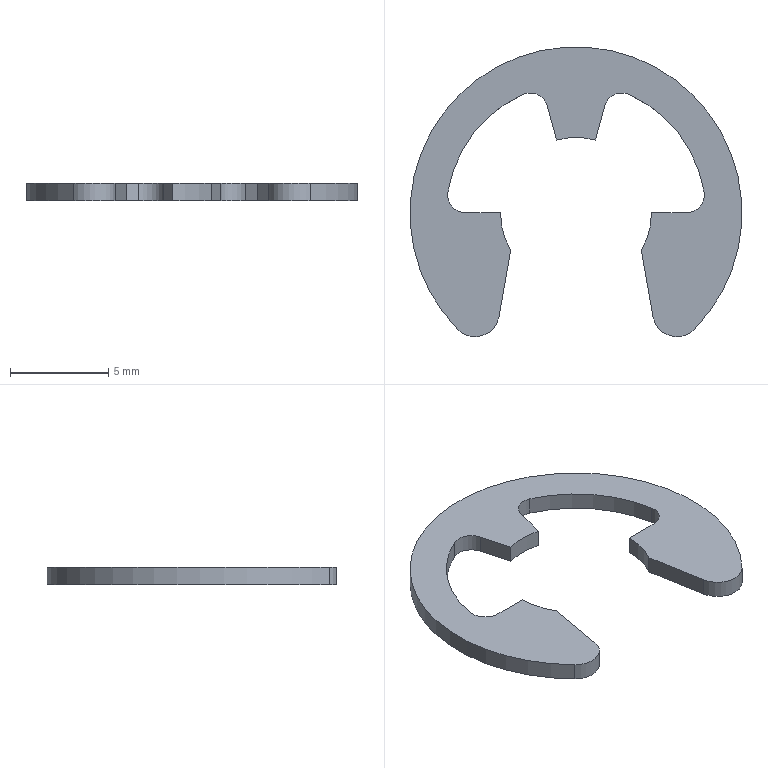Part | SolidWorks | features BaseBody 1 | 1 solid | 20 faces | box 16.932 x 14.78 x 0.889 mm | volume 89.694 mm3 | cylinder 12 | plane 8 | commonest cylinder face diameters 1.829 x4 7.696 x3 2.475 x2 13.237 x2 16.932 x1
STEP:
#1=CARTESIAN_POINT('',(5.631,0.,0.));
#2=VERTEX_POINT('',#1);
#3=CARTESIAN_POINT('',(6.533,1.061,0.));
#4=VERTEX_POINT('',#3);
#5=CARTESIAN_POINT('',(5.631,0.9143,0.));
#6=DIRECTION('',(0.,0.,1.));
#7=DIRECTION('',(0.,-1.,0.));
#8=AXIS2_PLACEMENT_3D('',#5,#6,#7);
#9=CIRCLE('',#8,0.9143);
#10=EDGE_CURVE('',#2,#4,#9,.T.);
#11=ORIENTED_EDGE('',*,*,#10,.F.);
#12=CARTESIAN_POINT('',(3.848,0.,0.));
#13=VERTEX_POINT('',#12);
#14=CARTESIAN_POINT('',(3.848,0.,0.));
#15=DIRECTION('',(1.,0.,0.));
#16=VECTOR('',#15,1000.);
#17=LINE('',#14,#16);
#18=EDGE_CURVE('',#13,#2,#17,.T.);
#19=ORIENTED_EDGE('',*,*,#18,.F.);
#20=CARTESIAN_POINT('',(3.333,-1.924,0.));
#21=VERTEX_POINT('',#20);
#22=CARTESIAN_POINT('',(0.,0.,0.));
#23=DIRECTION('',(0.,0.,1.));
#24=DIRECTION('',(0.866,-0.5,0.));
#25=AXIS2_PLACEMENT_3D('',#22,#23,#24);
#26=CIRCLE('',#25,3.848);
#27=EDGE_CURVE('',#21,#13,#26,.T.);
#28=ORIENTED_EDGE('',*,*,#27,.F.);
#29=CARTESIAN_POINT('',(3.926,-5.292,0.));
#30=VERTEX_POINT('',#29);
#31=CARTESIAN_POINT('',(3.926,-5.292,0.));
#32=DIRECTION('',(-0.1736,0.9848,0.));
#33=VECTOR('',#32,1000.);
#34=LINE('',#31,#33);
#35=EDGE_CURVE('',#30,#21,#34,.T.);
#36=ORIENTED_EDGE('',*,*,#35,.F.);
#37=CARTESIAN_POINT('',(6.026,-5.946,0.));
#38=VERTEX_POINT('',#37);
#39=CARTESIAN_POINT('',(5.145,-5.077,0.));
#40=DIRECTION('',(0.,0.,-1.));
#41=DIRECTION('',(0.7118,-0.7024,0.));
#42=AXIS2_PLACEMENT_3D('',#39,#40,#41);
#43=CIRCLE('',#42,1.238);
#44=EDGE_CURVE('',#38,#30,#43,.T.);
#45=ORIENTED_EDGE('',*,*,#44,.F.);
#46=CARTESIAN_POINT('',(-6.026,-5.946,0.));
#47=VERTEX_POINT('',#46);
#48=CARTESIAN_POINT('',(0.,0.,0.));
#49=DIRECTION('',(0.,0.,-1.));
#50=DIRECTION('',(-0.7118,-0.7024,0.));
#51=AXIS2_PLACEMENT_3D('',#48,#49,#50);
#52=CIRCLE('',#51,8.466);
#53=EDGE_CURVE('',#47,#38,#52,.T.);
#54=ORIENTED_EDGE('',*,*,#53,.F.);
#55=CARTESIAN_POINT('',(-3.926,-5.292,0.));
#56=VERTEX_POINT('',#55);
#57=CARTESIAN_POINT('',(-5.145,-5.077,0.));
#58=DIRECTION('',(0.,0.,-1.));
#59=DIRECTION('',(0.9848,-0.1736,0.));
#60=AXIS2_PLACEMENT_3D('',#57,#58,#59);
#61=CIRCLE('',#60,1.238);
#62=EDGE_CURVE('',#56,#47,#61,.T.);
#63=ORIENTED_EDGE('',*,*,#62,.F.);
#64=CARTESIAN_POINT('',(-3.333,-1.924,0.));
#65=VERTEX_POINT('',#64);
#66=CARTESIAN_POINT('',(-3.333,-1.924,0.));
#67=DIRECTION('',(-0.1736,-0.9848,0.));
#68=VECTOR('',#67,1000.);
#69=LINE('',#66,#68);
#70=EDGE_CURVE('',#65,#56,#69,.T.);
#71=ORIENTED_EDGE('',*,*,#70,.F.);
#72=CARTESIAN_POINT('',(-3.848,0.,0.));
#73=VERTEX_POINT('',#72);
#74=CARTESIAN_POINT('',(0.,0.,0.));
#75=DIRECTION('',(0.,0.,1.));
#76=DIRECTION('',(-1.,0.,0.));
#77=AXIS2_PLACEMENT_3D('',#74,#75,#76);
#78=CIRCLE('',#77,3.848);
#79=EDGE_CURVE('',#73,#65,#78,.T.);
#80=ORIENTED_EDGE('',*,*,#79,.F.);
#81=CARTESIAN_POINT('',(-5.631,0.,0.));
#82=VERTEX_POINT('',#81);
#83=CARTESIAN_POINT('',(-5.631,0.,0.));
#84=DIRECTION('',(1.,0.,0.));
#85=VECTOR('',#84,1000.);
#86=LINE('',#83,#85);
#87=EDGE_CURVE('',#82,#73,#86,.T.);
#88=ORIENTED_EDGE('',*,*,#87,.F.);
#89=CARTESIAN_POINT('',(-6.533,1.061,0.));
#90=VERTEX_POINT('',#89);
#91=CARTESIAN_POINT('',(-5.631,0.9143,0.));
#92=DIRECTION('',(0.,0.,1.));
#93=DIRECTION('',(-0.9871,0.1603,0.));
#94=AXIS2_PLACEMENT_3D('',#91,#92,#93);
#95=CIRCLE('',#94,0.9143);
#96=EDGE_CURVE('',#90,#82,#95,.T.);
#97=ORIENTED_EDGE('',*,*,#96,.F.);
#98=CARTESIAN_POINT('',(-2.716,6.036,0.));
#99=VERTEX_POINT('',#98);
#100=CARTESIAN_POINT('',(0.,0.,0.));
#101=DIRECTION('',(0.,0.,1.));
#102=DIRECTION('',(-0.4103,0.912,0.));
#103=AXIS2_PLACEMENT_3D('',#100,#101,#102);
#104=CIRCLE('',#103,6.619);
#105=EDGE_CURVE('',#99,#90,#104,.T.);
#106=ORIENTED_EDGE('',*,*,#105,.F.);
#107=CARTESIAN_POINT('',(-1.457,5.439,0.));
#108=VERTEX_POINT('',#107);
#109=CARTESIAN_POINT('',(-2.34,5.202,0.));
#110=DIRECTION('',(0.,0.,1.));
#111=DIRECTION('',(0.9659,0.2588,0.));
#112=AXIS2_PLACEMENT_3D('',#109,#110,#111);
#113=CIRCLE('',#112,0.9143);
#114=EDGE_CURVE('',#108,#99,#113,.T.);
#115=ORIENTED_EDGE('',*,*,#114,.F.);
#116=CARTESIAN_POINT('',(-0.996,3.717,0.));
#117=VERTEX_POINT('',#116);
#118=CARTESIAN_POINT('',(-0.996,3.717,0.));
#119=DIRECTION('',(-0.2588,0.9659,0.));
#120=VECTOR('',#119,1000.);
#121=LINE('',#118,#120);
#122=EDGE_CURVE('',#117,#108,#121,.T.);
#123=ORIENTED_EDGE('',*,*,#122,.F.);
#124=CARTESIAN_POINT('',(0.996,3.717,0.));
#125=VERTEX_POINT('',#124);
#126=CARTESIAN_POINT('',(0.,0.,0.));
#127=DIRECTION('',(0.,0.,1.));
#128=DIRECTION('',(0.2588,0.9659,0.));
#129=AXIS2_PLACEMENT_3D('',#126,#127,#128);
#130=CIRCLE('',#129,3.848);
#131=EDGE_CURVE('',#125,#117,#130,.T.);
#132=ORIENTED_EDGE('',*,*,#131,.F.);
#133=CARTESIAN_POINT('',(1.457,5.439,0.));
#134=VERTEX_POINT('',#133);
#135=CARTESIAN_POINT('',(1.457,5.439,0.));
#136=DIRECTION('',(-0.2588,-0.9659,0.));
#137=VECTOR('',#136,1000.);
#138=LINE('',#135,#137);
#139=EDGE_CURVE('',#134,#125,#138,.T.);
#140=ORIENTED_EDGE('',*,*,#139,.F.);
#141=CARTESIAN_POINT('',(2.716,6.036,0.));
#142=VERTEX_POINT('',#141);
#143=CARTESIAN_POINT('',(2.34,5.202,0.));
#144=DIRECTION('',(0.,0.,1.));
#145=DIRECTION('',(0.4103,0.912,0.));
#146=AXIS2_PLACEMENT_3D('',#143,#144,#145);
#147=CIRCLE('',#146,0.9143);
#148=EDGE_CURVE('',#142,#134,#147,.T.);
#149=ORIENTED_EDGE('',*,*,#148,.F.);
#150=CARTESIAN_POINT('',(0.,0.,0.));
#151=DIRECTION('',(0.,0.,1.));
#152=DIRECTION('',(0.9871,0.1603,0.));
#153=AXIS2_PLACEMENT_3D('',#150,#151,#152);
#154=CIRCLE('',#153,6.619);
#155=EDGE_CURVE('',#4,#142,#154,.T.);
#156=ORIENTED_EDGE('',*,*,#155,.F.);
#157=EDGE_LOOP('',(#11,#19,#28,#36,#45,#54,#63,#71,#80,#88,#97,#106,#115,#123,#132,#140,#149,#156));
#158=FACE_OUTER_BOUND('',#157,.T.);
#159=CARTESIAN_POINT('',(5.631,0.9143,0.));
#160=DIRECTION('',(0.,0.,1.));
#161=DIRECTION('',(1.,0.,0.));
#162=AXIS2_PLACEMENT_3D('',#159,#160,#161);
#163=PLANE('',#162);
#164=ADVANCED_FACE('',(#158),#163,.T.);
#165=CARTESIAN_POINT('',(6.533,1.061,-0.889));
#166=VERTEX_POINT('',#165);
#167=CARTESIAN_POINT('',(5.631,0.,-0.889));
#168=VERTEX_POINT('',#167);
#169=CARTESIAN_POINT('',(5.631,0.9143,-0.889));
#170=DIRECTION('',(0.,0.,-1.));
#171=DIRECTION('',(0.9871,0.1603,0.));
#172=AXIS2_PLACEMENT_3D('',#169,#170,#171);
#173=CIRCLE('',#172,0.9143);
#174=EDGE_CURVE('',#166,#168,#173,.T.);
#175=ORIENTED_EDGE('',*,*,#174,.F.);
#176=CARTESIAN_POINT('',(2.716,6.036,-0.889));
#177=VERTEX_POINT('',#176);
#178=CARTESIAN_POINT('',(0.,0.,-0.889));
#179=DIRECTION('',(0.,0.,-1.));
#180=DIRECTION('',(0.4103,0.912,0.));
#181=AXIS2_PLACEMENT_3D('',#178,#179,#180);
#182=CIRCLE('',#181,6.619);
#183=EDGE_CURVE('',#177,#166,#182,.T.);
#184=ORIENTED_EDGE('',*,*,#183,.F.);
#185=CARTESIAN_POINT('',(1.457,5.439,-0.889));
#186=VERTEX_POINT('',#185);
#187=CARTESIAN_POINT('',(2.34,5.202,-0.889));
#188=DIRECTION('',(0.,0.,-1.));
#189=DIRECTION('',(-0.9659,0.2588,0.));
#190=AXIS2_PLACEMENT_3D('',#187,#188,#189);
#191=CIRCLE('',#190,0.9143);
#192=EDGE_CURVE('',#186,#177,#191,.T.);
#193=ORIENTED_EDGE('',*,*,#192,.F.);
#194=CARTESIAN_POINT('',(0.996,3.717,-0.889));
#195=VERTEX_POINT('',#194);
#196=CARTESIAN_POINT('',(0.996,3.717,-0.889));
#197=DIRECTION('',(0.2588,0.9659,0.));
#198=VECTOR('',#197,1000.);
#199=LINE('',#196,#198);
#200=EDGE_CURVE('',#195,#186,#199,.T.);
#201=ORIENTED_EDGE('',*,*,#200,.F.);
#202=CARTESIAN_POINT('',(-0.996,3.717,-0.889));
#203=VERTEX_POINT('',#202);
#204=CARTESIAN_POINT('',(0.,0.,-0.889));
#205=DIRECTION('',(0.,0.,-1.));
#206=DIRECTION('',(-0.2588,0.9659,0.));
#207=AXIS2_PLACEMENT_3D('',#204,#205,#206);
#208=CIRCLE('',#207,3.848);
#209=EDGE_CURVE('',#203,#195,#208,.T.);
#210=ORIENTED_EDGE('',*,*,#209,.F.);
#211=CARTESIAN_POINT('',(-1.457,5.439,-0.889));
#212=VERTEX_POINT('',#211);
#213=CARTESIAN_POINT('',(-1.457,5.439,-0.889));
#214=DIRECTION('',(0.2588,-0.9659,0.));
#215=VECTOR('',#214,1000.);
#216=LINE('',#213,#215);
#217=EDGE_CURVE('',#212,#203,#216,.T.);
#218=ORIENTED_EDGE('',*,*,#217,.F.);
#219=CARTESIAN_POINT('',(-2.716,6.036,-0.889));
#220=VERTEX_POINT('',#219);
#221=CARTESIAN_POINT('',(-2.34,5.202,-0.889));
#222=DIRECTION('',(0.,0.,-1.));
#223=DIRECTION('',(-0.4103,0.912,0.));
#224=AXIS2_PLACEMENT_3D('',#221,#222,#223);
#225=CIRCLE('',#224,0.9143);
#226=EDGE_CURVE('',#220,#212,#225,.T.);
#227=ORIENTED_EDGE('',*,*,#226,.F.);
#228=CARTESIAN_POINT('',(-6.533,1.061,-0.889));
#229=VERTEX_POINT('',#228);
#230=CARTESIAN_POINT('',(0.,0.,-0.889));
#231=DIRECTION('',(0.,0.,-1.));
#232=DIRECTION('',(-0.9871,0.1603,0.));
#233=AXIS2_PLACEMENT_3D('',#230,#231,#232);
#234=CIRCLE('',#233,6.619);
#235=EDGE_CURVE('',#229,#220,#234,.T.);
#236=ORIENTED_EDGE('',*,*,#235,.F.);
#237=CARTESIAN_POINT('',(-5.631,0.,-0.889));
#238=VERTEX_POINT('',#237);
#239=CARTESIAN_POINT('',(-5.631,0.9143,-0.889));
#240=DIRECTION('',(0.,0.,-1.));
#241=DIRECTION('',(0.,-1.,0.));
#242=AXIS2_PLACEMENT_3D('',#239,#240,#241);
#243=CIRCLE('',#242,0.9143);
#244=EDGE_CURVE('',#238,#229,#243,.T.);
#245=ORIENTED_EDGE('',*,*,#244,.F.);
#246=CARTESIAN_POINT('',(-3.848,0.,-0.889));
#247=VERTEX_POINT('',#246);
#248=CARTESIAN_POINT('',(-3.848,0.,-0.889));
#249=DIRECTION('',(-1.,0.,0.));
#250=VECTOR('',#249,1000.);
#251=LINE('',#248,#250);
#252=EDGE_CURVE('',#247,#238,#251,.T.);
#253=ORIENTED_EDGE('',*,*,#252,.F.);
#254=CARTESIAN_POINT('',(-3.333,-1.924,-0.889));
#255=VERTEX_POINT('',#254);
#256=CARTESIAN_POINT('',(0.,0.,-0.889));
#257=DIRECTION('',(0.,0.,-1.));
#258=DIRECTION('',(-0.866,-0.5,0.));
#259=AXIS2_PLACEMENT_3D('',#256,#257,#258);
#260=CIRCLE('',#259,3.848);
#261=EDGE_CURVE('',#255,#247,#260,.T.);
#262=ORIENTED_EDGE('',*,*,#261,.F.);
#263=CARTESIAN_POINT('',(-3.926,-5.292,-0.889));
#264=VERTEX_POINT('',#263);
#265=CARTESIAN_POINT('',(-3.926,-5.292,-0.889));
#266=DIRECTION('',(0.1736,0.9848,0.));
#267=VECTOR('',#266,1000.);
#268=LINE('',#265,#267);
#269=EDGE_CURVE('',#264,#255,#268,.T.);
#270=ORIENTED_EDGE('',*,*,#269,.F.);
#271=CARTESIAN_POINT('',(-6.026,-5.946,-0.889));
#272=VERTEX_POINT('',#271);
#273=CARTESIAN_POINT('',(-5.145,-5.077,-0.889));
#274=DIRECTION('',(0.,0.,1.));
#275=DIRECTION('',(-0.7118,-0.7024,0.));
#276=AXIS2_PLACEMENT_3D('',#273,#274,#275);
#277=CIRCLE('',#276,1.238);
#278=EDGE_CURVE('',#272,#264,#277,.T.);
#279=ORIENTED_EDGE('',*,*,#278,.F.);
#280=CARTESIAN_POINT('',(6.026,-5.946,-0.889));
#281=VERTEX_POINT('',#280);
#282=CARTESIAN_POINT('',(0.,0.,-0.889));
#283=DIRECTION('',(0.,0.,1.));
#284=DIRECTION('',(0.7118,-0.7024,0.));
#285=AXIS2_PLACEMENT_3D('',#282,#283,#284);
#286=CIRCLE('',#285,8.466);
#287=EDGE_CURVE('',#281,#272,#286,.T.);
#288=ORIENTED_EDGE('',*,*,#287,.F.);
#289=CARTESIAN_POINT('',(3.926,-5.292,-0.889));
#290=VERTEX_POINT('',#289);
#291=CARTESIAN_POINT('',(5.145,-5.077,-0.889));
#292=DIRECTION('',(0.,0.,1.));
#293=DIRECTION('',(-0.9848,-0.1736,0.));
#294=AXIS2_PLACEMENT_3D('',#291,#292,#293);
#295=CIRCLE('',#294,1.238);
#296=EDGE_CURVE('',#290,#281,#295,.T.);
#297=ORIENTED_EDGE('',*,*,#296,.F.);
#298=CARTESIAN_POINT('',(3.333,-1.924,-0.889));
#299=VERTEX_POINT('',#298);
#300=CARTESIAN_POINT('',(3.333,-1.924,-0.889));
#301=DIRECTION('',(0.1736,-0.9848,0.));
#302=VECTOR('',#301,1000.);
#303=LINE('',#300,#302);
#304=EDGE_CURVE('',#299,#290,#303,.T.);
#305=ORIENTED_EDGE('',*,*,#304,.F.);
#306=CARTESIAN_POINT('',(3.848,0.,-0.889));
#307=VERTEX_POINT('',#306);
#308=CARTESIAN_POINT('',(0.,0.,-0.889));
#309=DIRECTION('',(0.,0.,-1.));
#310=DIRECTION('',(1.,0.,0.));
#311=AXIS2_PLACEMENT_3D('',#308,#309,#310);
#312=CIRCLE('',#311,3.848);
#313=EDGE_CURVE('',#307,#299,#312,.T.);
#314=ORIENTED_EDGE('',*,*,#313,.F.);
#315=CARTESIAN_POINT('',(5.631,0.,-0.889));
#316=DIRECTION('',(-1.,0.,0.));
#317=VECTOR('',#316,1000.);
#318=LINE('',#315,#317);
#319=EDGE_CURVE('',#168,#307,#318,.T.);
#320=ORIENTED_EDGE('',*,*,#319,.F.);
#321=EDGE_LOOP('',(#175,#184,#193,#201,#210,#218,#227,#236,#245,#253,#262,#270,#279,#288,#297,#305,#314,#320));
#322=FACE_OUTER_BOUND('',#321,.T.);
#323=CARTESIAN_POINT('',(5.631,0.9143,-0.889));
#324=DIRECTION('',(0.,0.,-1.));
#325=DIRECTION('',(0.,-1.,0.));
#326=AXIS2_PLACEMENT_3D('',#323,#324,#325);
#327=PLANE('',#326);
#328=ADVANCED_FACE('',(#322),#327,.T.);
#329=ORIENTED_EDGE('',*,*,#18,.T.);
#330=CARTESIAN_POINT('',(5.631,0.,-0.889));
#331=DIRECTION('',(0.,0.,1.));
#332=VECTOR('',#331,1000.);
#333=LINE('',#330,#332);
#334=EDGE_CURVE('',#168,#2,#333,.T.);
#335=ORIENTED_EDGE('',*,*,#334,.F.);
#336=ORIENTED_EDGE('',*,*,#319,.T.);
#337=CARTESIAN_POINT('',(3.848,0.,0.));
#338=DIRECTION('',(0.,0.,-1.));
#339=VECTOR('',#338,1000.);
#340=LINE('',#337,#339);
#341=EDGE_CURVE('',#13,#307,#340,.T.);
#342=ORIENTED_EDGE('',*,*,#341,.F.);
#343=EDGE_LOOP('',(#329,#335,#336,#342));
#344=FACE_OUTER_BOUND('',#343,.T.);
#345=CARTESIAN_POINT('',(3.848,0.,-0.889));
#346=DIRECTION('',(0.,1.,0.));
#347=DIRECTION('',(1.,0.,0.));
#348=AXIS2_PLACEMENT_3D('',#345,#346,#347);
#349=PLANE('',#348);
#350=ADVANCED_FACE('',(#344),#349,.T.);
#351=ORIENTED_EDGE('',*,*,#27,.T.);
#352=ORIENTED_EDGE('',*,*,#341,.T.);
#353=ORIENTED_EDGE('',*,*,#313,.T.);
#354=CARTESIAN_POINT('',(3.333,-1.924,0.));
#355=DIRECTION('',(0.,0.,-1.));
#356=VECTOR('',#355,1000.);
#357=LINE('',#354,#356);
#358=EDGE_CURVE('',#21,#299,#357,.T.);
#359=ORIENTED_EDGE('',*,*,#358,.F.);
#360=EDGE_LOOP('',(#351,#352,#353,#359));
#361=FACE_OUTER_BOUND('',#360,.T.);
#362=CARTESIAN_POINT('',(0.,0.,-0.889));
#363=DIRECTION('',(0.,0.,1.));
#364=DIRECTION('',(0.866,-0.5,0.));
#365=AXIS2_PLACEMENT_3D('',#362,#363,#364);
#366=CYLINDRICAL_SURFACE('',#365,3.848);
#367=ADVANCED_FACE('',(#361),#366,.F.);
#368=ORIENTED_EDGE('',*,*,#35,.T.);
#369=ORIENTED_EDGE('',*,*,#358,.T.);
#370=ORIENTED_EDGE('',*,*,#304,.T.);
#371=CARTESIAN_POINT('',(3.926,-5.292,0.));
#372=DIRECTION('',(0.,0.,-1.));
#373=VECTOR('',#372,1000.);
#374=LINE('',#371,#373);
#375=EDGE_CURVE('',#30,#290,#374,.T.);
#376=ORIENTED_EDGE('',*,*,#375,.F.);
#377=EDGE_LOOP('',(#368,#369,#370,#376));
#378=FACE_OUTER_BOUND('',#377,.T.);
#379=CARTESIAN_POINT('',(3.333,-1.924,-0.889));
#380=DIRECTION('',(-0.9848,-0.1736,0.));
#381=DIRECTION('',(-0.1736,0.9848,0.));
#382=AXIS2_PLACEMENT_3D('',#379,#380,#381);
#383=PLANE('',#382);
#384=ADVANCED_FACE('',(#378),#383,.T.);
#385=ORIENTED_EDGE('',*,*,#44,.T.);
#386=ORIENTED_EDGE('',*,*,#375,.T.);
#387=ORIENTED_EDGE('',*,*,#296,.T.);
#388=CARTESIAN_POINT('',(6.026,-5.946,0.));
#389=DIRECTION('',(0.,0.,-1.));
#390=VECTOR('',#389,1000.);
#391=LINE('',#388,#390);
#392=EDGE_CURVE('',#38,#281,#391,.T.);
#393=ORIENTED_EDGE('',*,*,#392,.F.);
#394=EDGE_LOOP('',(#385,#386,#387,#393));
#395=FACE_OUTER_BOUND('',#394,.T.);
#396=CARTESIAN_POINT('',(5.145,-5.077,-0.889));
#397=DIRECTION('',(0.,0.,1.));
#398=DIRECTION('',(0.7118,-0.7024,0.));
#399=AXIS2_PLACEMENT_3D('',#396,#397,#398);
#400=CYLINDRICAL_SURFACE('',#399,1.238);
#401=ADVANCED_FACE('',(#395),#400,.T.);
#402=ORIENTED_EDGE('',*,*,#53,.T.);
#403=ORIENTED_EDGE('',*,*,#392,.T.);
#404=ORIENTED_EDGE('',*,*,#287,.T.);
#405=CARTESIAN_POINT('',(-6.026,-5.946,0.));
#406=DIRECTION('',(0.,0.,-1.));
#407=VECTOR('',#406,1000.);
#408=LINE('',#405,#407);
#409=EDGE_CURVE('',#47,#272,#408,.T.);
#410=ORIENTED_EDGE('',*,*,#409,.F.);
#411=EDGE_LOOP('',(#402,#403,#404,#410));
#412=FACE_OUTER_BOUND('',#411,.T.);
#413=CARTESIAN_POINT('',(0.,0.,-0.889));
#414=DIRECTION('',(0.,0.,1.));
#415=DIRECTION('',(-0.7118,-0.7024,0.));
#416=AXIS2_PLACEMENT_3D('',#413,#414,#415);
#417=CYLINDRICAL_SURFACE('',#416,8.466);
#418=ADVANCED_FACE('',(#412),#417,.T.);
#419=ORIENTED_EDGE('',*,*,#62,.T.);
#420=ORIENTED_EDGE('',*,*,#409,.T.);
#421=ORIENTED_EDGE('',*,*,#278,.T.);
#422=CARTESIAN_POINT('',(-3.926,-5.292,0.));
#423=DIRECTION('',(0.,0.,-1.));
#424=VECTOR('',#423,1000.);
#425=LINE('',#422,#424);
#426=EDGE_CURVE('',#56,#264,#425,.T.);
#427=ORIENTED_EDGE('',*,*,#426,.F.);
#428=EDGE_LOOP('',(#419,#420,#421,#427));
#429=FACE_OUTER_BOUND('',#428,.T.);
#430=CARTESIAN_POINT('',(-5.145,-5.077,-0.889));
#431=DIRECTION('',(0.,0.,1.));
#432=DIRECTION('',(0.9848,-0.1736,0.));
#433=AXIS2_PLACEMENT_3D('',#430,#431,#432);
#434=CYLINDRICAL_SURFACE('',#433,1.238);
#435=ADVANCED_FACE('',(#429),#434,.T.);
#436=ORIENTED_EDGE('',*,*,#70,.T.);
#437=ORIENTED_EDGE('',*,*,#426,.T.);
#438=ORIENTED_EDGE('',*,*,#269,.T.);
#439=CARTESIAN_POINT('',(-3.333,-1.924,0.));
#440=DIRECTION('',(0.,0.,-1.));
#441=VECTOR('',#440,1000.);
#442=LINE('',#439,#441);
#443=EDGE_CURVE('',#65,#255,#442,.T.);
#444=ORIENTED_EDGE('',*,*,#443,.F.);
#445=EDGE_LOOP('',(#436,#437,#438,#444));
#446=FACE_OUTER_BOUND('',#445,.T.);
#447=CARTESIAN_POINT('',(-3.333,-1.924,-0.889));
#448=DIRECTION('',(0.9848,-0.1736,0.));
#449=DIRECTION('',(0.,0.,-1.));
#450=AXIS2_PLACEMENT_3D('',#447,#448,#449);
#451=PLANE('',#450);
#452=ADVANCED_FACE('',(#446),#451,.T.);
#453=ORIENTED_EDGE('',*,*,#79,.T.);
#454=ORIENTED_EDGE('',*,*,#443,.T.);
#455=ORIENTED_EDGE('',*,*,#261,.T.);
#456=CARTESIAN_POINT('',(-3.848,0.,0.));
#457=DIRECTION('',(0.,0.,-1.));
#458=VECTOR('',#457,1000.);
#459=LINE('',#456,#458);
#460=EDGE_CURVE('',#73,#247,#459,.T.);
#461=ORIENTED_EDGE('',*,*,#460,.F.);
#462=EDGE_LOOP('',(#453,#454,#455,#461));
#463=FACE_OUTER_BOUND('',#462,.T.);
#464=CARTESIAN_POINT('',(0.,0.,-0.889));
#465=DIRECTION('',(0.,0.,1.));
#466=DIRECTION('',(-1.,0.,0.));
#467=AXIS2_PLACEMENT_3D('',#464,#465,#466);
#468=CYLINDRICAL_SURFACE('',#467,3.848);
#469=ADVANCED_FACE('',(#463),#468,.F.);
#470=ORIENTED_EDGE('',*,*,#87,.T.);
#471=ORIENTED_EDGE('',*,*,#460,.T.);
#472=ORIENTED_EDGE('',*,*,#252,.T.);
#473=CARTESIAN_POINT('',(-5.631,0.,0.));
#474=DIRECTION('',(0.,0.,-1.));
#475=VECTOR('',#474,1000.);
#476=LINE('',#473,#475);
#477=EDGE_CURVE('',#82,#238,#476,.T.);
#478=ORIENTED_EDGE('',*,*,#477,.F.);
#479=EDGE_LOOP('',(#470,#471,#472,#478));
#480=FACE_OUTER_BOUND('',#479,.T.);
#481=CARTESIAN_POINT('',(-3.848,0.,-0.889));
#482=DIRECTION('',(0.,1.,0.));
#483=DIRECTION('',(1.,0.,0.));
#484=AXIS2_PLACEMENT_3D('',#481,#482,#483);
#485=PLANE('',#484);
#486=ADVANCED_FACE('',(#480),#485,.T.);
#487=ORIENTED_EDGE('',*,*,#96,.T.);
#488=ORIENTED_EDGE('',*,*,#477,.T.);
#489=ORIENTED_EDGE('',*,*,#244,.T.);
#490=CARTESIAN_POINT('',(-6.533,1.061,0.));
#491=DIRECTION('',(0.,0.,-1.));
#492=VECTOR('',#491,1000.);
#493=LINE('',#490,#492);
#494=EDGE_CURVE('',#90,#229,#493,.T.);
#495=ORIENTED_EDGE('',*,*,#494,.F.);
#496=EDGE_LOOP('',(#487,#488,#489,#495));
#497=FACE_OUTER_BOUND('',#496,.T.);
#498=CARTESIAN_POINT('',(-5.631,0.9143,-0.889));
#499=DIRECTION('',(0.,0.,1.));
#500=DIRECTION('',(-0.9871,0.1603,0.));
#501=AXIS2_PLACEMENT_3D('',#498,#499,#500);
#502=CYLINDRICAL_SURFACE('',#501,0.9143);
#503=ADVANCED_FACE('',(#497),#502,.F.);
#504=ORIENTED_EDGE('',*,*,#105,.T.);
#505=ORIENTED_EDGE('',*,*,#494,.T.);
#506=ORIENTED_EDGE('',*,*,#235,.T.);
#507=CARTESIAN_POINT('',(-2.716,6.036,0.));
#508=DIRECTION('',(0.,0.,-1.));
#509=VECTOR('',#508,1000.);
#510=LINE('',#507,#509);
#511=EDGE_CURVE('',#99,#220,#510,.T.);
#512=ORIENTED_EDGE('',*,*,#511,.F.);
#513=EDGE_LOOP('',(#504,#505,#506,#512));
#514=FACE_OUTER_BOUND('',#513,.T.);
#515=CARTESIAN_POINT('',(0.,0.,-0.889));
#516=DIRECTION('',(0.,0.,1.));
#517=DIRECTION('',(-0.4103,0.912,0.));
#518=AXIS2_PLACEMENT_3D('',#515,#516,#517);
#519=CYLINDRICAL_SURFACE('',#518,6.619);
#520=ADVANCED_FACE('',(#514),#519,.F.);
#521=ORIENTED_EDGE('',*,*,#114,.T.);
#522=ORIENTED_EDGE('',*,*,#511,.T.);
#523=ORIENTED_EDGE('',*,*,#226,.T.);
#524=CARTESIAN_POINT('',(-1.457,5.439,0.));
#525=DIRECTION('',(0.,0.,-1.));
#526=VECTOR('',#525,1000.);
#527=LINE('',#524,#526);
#528=EDGE_CURVE('',#108,#212,#527,.T.);
#529=ORIENTED_EDGE('',*,*,#528,.F.);
#530=EDGE_LOOP('',(#521,#522,#523,#529));
#531=FACE_OUTER_BOUND('',#530,.T.);
#532=CARTESIAN_POINT('',(-2.34,5.202,-0.889));
#533=DIRECTION('',(0.,0.,1.));
#534=DIRECTION('',(0.9659,0.2588,0.));
#535=AXIS2_PLACEMENT_3D('',#532,#533,#534);
#536=CYLINDRICAL_SURFACE('',#535,0.9143);
#537=ADVANCED_FACE('',(#531),#536,.F.);
#538=ORIENTED_EDGE('',*,*,#122,.T.);
#539=ORIENTED_EDGE('',*,*,#528,.T.);
#540=ORIENTED_EDGE('',*,*,#217,.T.);
#541=CARTESIAN_POINT('',(-0.996,3.717,0.));
#542=DIRECTION('',(0.,0.,-1.));
#543=VECTOR('',#542,1000.);
#544=LINE('',#541,#543);
#545=EDGE_CURVE('',#117,#203,#544,.T.);
#546=ORIENTED_EDGE('',*,*,#545,.F.);
#547=EDGE_LOOP('',(#538,#539,#540,#546));
#548=FACE_OUTER_BOUND('',#547,.T.);
#549=CARTESIAN_POINT('',(-0.996,3.717,-0.889));
#550=DIRECTION('',(-0.9659,-0.2588,0.));
#551=DIRECTION('',(-0.2588,0.9659,0.));
#552=AXIS2_PLACEMENT_3D('',#549,#550,#551);
#553=PLANE('',#552);
#554=ADVANCED_FACE('',(#548),#553,.T.);
#555=ORIENTED_EDGE('',*,*,#131,.T.);
#556=ORIENTED_EDGE('',*,*,#545,.T.);
#557=ORIENTED_EDGE('',*,*,#209,.T.);
#558=CARTESIAN_POINT('',(0.996,3.717,0.));
#559=DIRECTION('',(0.,0.,-1.));
#560=VECTOR('',#559,1000.);
#561=LINE('',#558,#560);
#562=EDGE_CURVE('',#125,#195,#561,.T.);
#563=ORIENTED_EDGE('',*,*,#562,.F.);
#564=EDGE_LOOP('',(#555,#556,#557,#563));
#565=FACE_OUTER_BOUND('',#564,.T.);
#566=CARTESIAN_POINT('',(0.,0.,-0.889));
#567=DIRECTION('',(0.,0.,1.));
#568=DIRECTION('',(0.2588,0.9659,0.));
#569=AXIS2_PLACEMENT_3D('',#566,#567,#568);
#570=CYLINDRICAL_SURFACE('',#569,3.848);
#571=ADVANCED_FACE('',(#565),#570,.F.);
#572=ORIENTED_EDGE('',*,*,#139,.T.);
#573=ORIENTED_EDGE('',*,*,#562,.T.);
#574=ORIENTED_EDGE('',*,*,#200,.T.);
#575=CARTESIAN_POINT('',(1.457,5.439,0.));
#576=DIRECTION('',(0.,0.,-1.));
#577=VECTOR('',#576,1000.);
#578=LINE('',#575,#577);
#579=EDGE_CURVE('',#134,#186,#578,.T.);
#580=ORIENTED_EDGE('',*,*,#579,.F.);
#581=EDGE_LOOP('',(#572,#573,#574,#580));
#582=FACE_OUTER_BOUND('',#581,.T.);
#583=CARTESIAN_POINT('',(0.996,3.717,-0.889));
#584=DIRECTION('',(0.9659,-0.2588,0.));
#585=DIRECTION('',(0.,0.,-1.));
#586=AXIS2_PLACEMENT_3D('',#583,#584,#585);
#587=PLANE('',#586);
#588=ADVANCED_FACE('',(#582),#587,.T.);
#589=ORIENTED_EDGE('',*,*,#148,.T.);
#590=ORIENTED_EDGE('',*,*,#579,.T.);
#591=ORIENTED_EDGE('',*,*,#192,.T.);
#592=CARTESIAN_POINT('',(2.716,6.036,0.));
#593=DIRECTION('',(0.,0.,-1.));
#594=VECTOR('',#593,1000.);
#595=LINE('',#592,#594);
#596=EDGE_CURVE('',#142,#177,#595,.T.);
#597=ORIENTED_EDGE('',*,*,#596,.F.);
#598=EDGE_LOOP('',(#589,#590,#591,#597));
#599=FACE_OUTER_BOUND('',#598,.T.);
#600=CARTESIAN_POINT('',(2.34,5.202,-0.889));
#601=DIRECTION('',(0.,0.,1.));
#602=DIRECTION('',(0.4103,0.912,0.));
#603=AXIS2_PLACEMENT_3D('',#600,#601,#602);
#604=CYLINDRICAL_SURFACE('',#603,0.9143);
#605=ADVANCED_FACE('',(#599),#604,.F.);
#606=ORIENTED_EDGE('',*,*,#155,.T.);
#607=ORIENTED_EDGE('',*,*,#596,.T.);
#608=ORIENTED_EDGE('',*,*,#183,.T.);
#609=CARTESIAN_POINT('',(6.533,1.061,0.));
#610=DIRECTION('',(0.,0.,-1.));
#611=VECTOR('',#610,1000.);
#612=LINE('',#609,#611);
#613=EDGE_CURVE('',#4,#166,#612,.T.);
#614=ORIENTED_EDGE('',*,*,#613,.F.);
#615=EDGE_LOOP('',(#606,#607,#608,#614));
#616=FACE_OUTER_BOUND('',#615,.T.);
#617=CARTESIAN_POINT('',(0.,0.,-0.889));
#618=DIRECTION('',(0.,0.,1.));
#619=DIRECTION('',(0.9871,0.1603,0.));
#620=AXIS2_PLACEMENT_3D('',#617,#618,#619);
#621=CYLINDRICAL_SURFACE('',#620,6.619);
#622=ADVANCED_FACE('',(#616),#621,.F.);
#623=ORIENTED_EDGE('',*,*,#10,.T.);
#624=ORIENTED_EDGE('',*,*,#613,.T.);
#625=ORIENTED_EDGE('',*,*,#174,.T.);
#626=ORIENTED_EDGE('',*,*,#334,.T.);
#627=EDGE_LOOP('',(#623,#624,#625,#626));
#628=FACE_OUTER_BOUND('',#627,.T.);
#629=CARTESIAN_POINT('',(5.631,0.9143,-0.889));
#630=DIRECTION('',(0.,0.,1.));
#631=DIRECTION('',(0.000000003,-1.,0.));
#632=AXIS2_PLACEMENT_3D('',#629,#630,#631);
#633=CYLINDRICAL_SURFACE('',#632,0.9143);
#634=ADVANCED_FACE('',(#628),#633,.F.);
#635=CLOSED_SHELL('',(#164,#328,#350,#367,#384,#401,#418,#435,#452,#469,#486,#503,#520,#537,#554,#571,#588,#605,#622,#634));
#636=MANIFOLD_SOLID_BREP('',#635);
#637=CARTESIAN_POINT('',(0.,0.,0.));
#638=DIRECTION('',(0.,0.,1.));
#639=DIRECTION('',(1.,0.,0.));
#640=AXIS2_PLACEMENT_3D('',#637,#638,#639);
#641=(LENGTH_UNIT()NAMED_UNIT(*)SI_UNIT(.MILLI.,.METRE.));
#642=UNCERTAINTY_MEASURE_WITH_UNIT(LENGTH_MEASURE(0.00001),#641,'','');
#643=(NAMED_UNIT(*)PLANE_ANGLE_UNIT()SI_UNIT($,.RADIAN.));
#644=(NAMED_UNIT(*)SI_UNIT($,.STERADIAN.)SOLID_ANGLE_UNIT());
#645=(GEOMETRIC_REPRESENTATION_CONTEXT(3)GLOBAL_UNCERTAINTY_ASSIGNED_CONTEXT((#642))GLOBAL_UNIT_ASSIGNED_CONTEXT((#641,#643,#644))REPRESENTATION_CONTEXT('',''));
#646=ADVANCED_BREP_SHAPE_REPRESENTATION('',(#636,#640),#645);